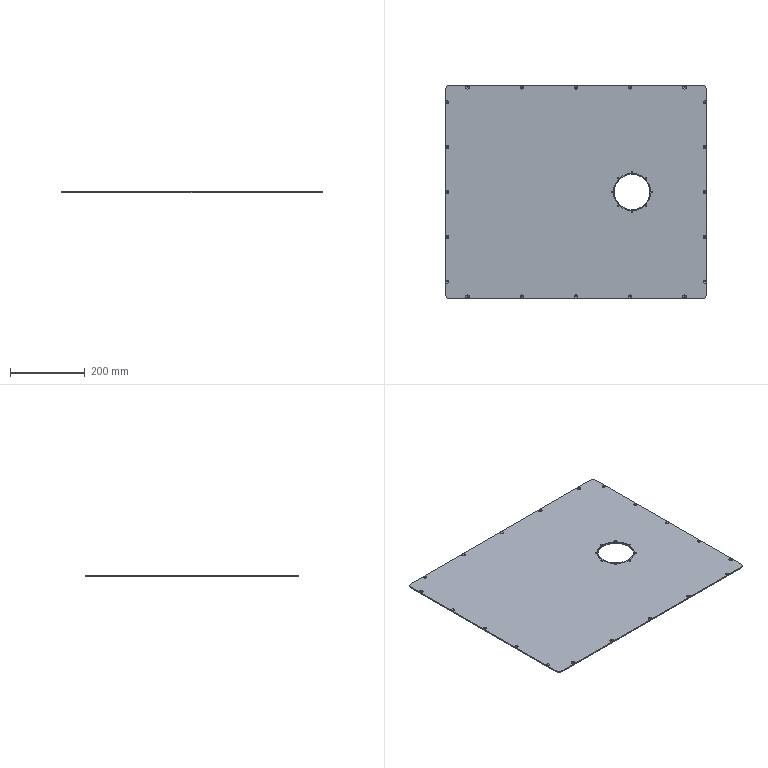Part | SolidWorks | features Cut 2, Extrusion 1, HoleWzd 1, ICE 1 | 1 solid | 114 faces | box 700 x 570 x 3 mm | volume 1172283 mm3 | cylinder 66 | cone 40 | plane 8 | commonest cylinder face diameters 4.5 x56 25 x4 95 x2 97 x2 100 x2